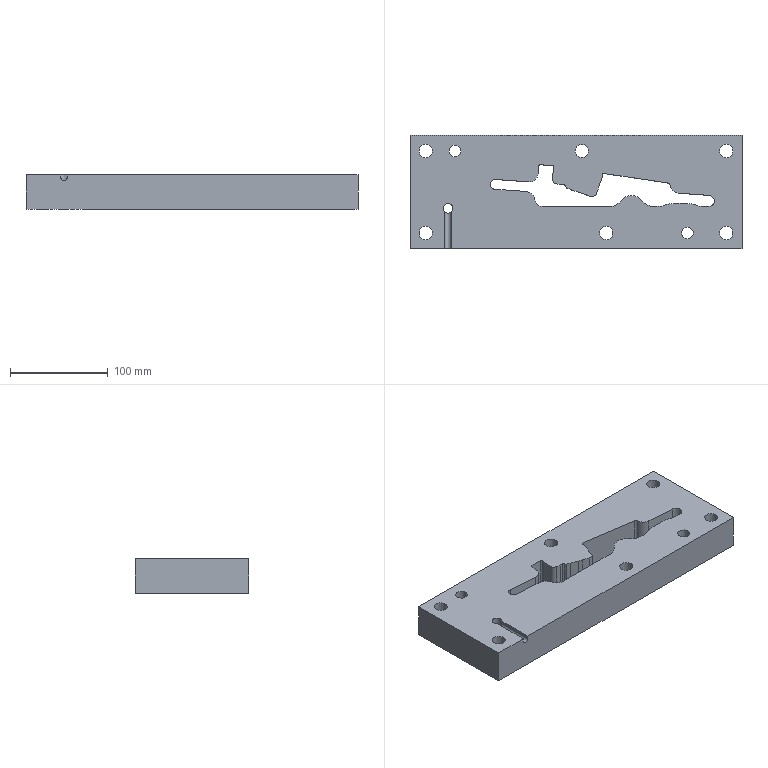Part | NX | features 7 2 | 1 solid | 113 faces | box 340 x 116 x 35 mm | volume 1137883 mm3 | cylinder 56 | plane 53 | cone 4 | commonest cylinder face diameters 10 x11 20 x7 2 x6 13.5 x6 6.799 x4 40 x4